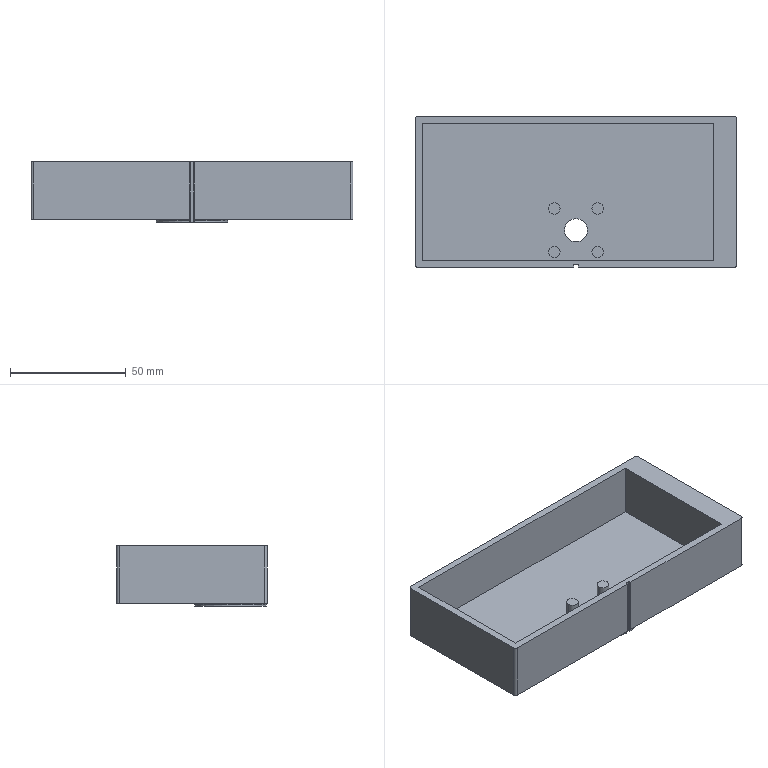Part | SolidWorks | features ICE 12, Fillet 3, Extrusion 1, Shell 1 | 1 solid | 76 faces | box 139 x 65 x 26.2 mm | volume 46705 mm3 | cylinder 33 | plane 32 | torus 11 | commonest cylinder face diameters 1 x8 5 x8 2 x4 31 x3 0.4 x2 10 x2